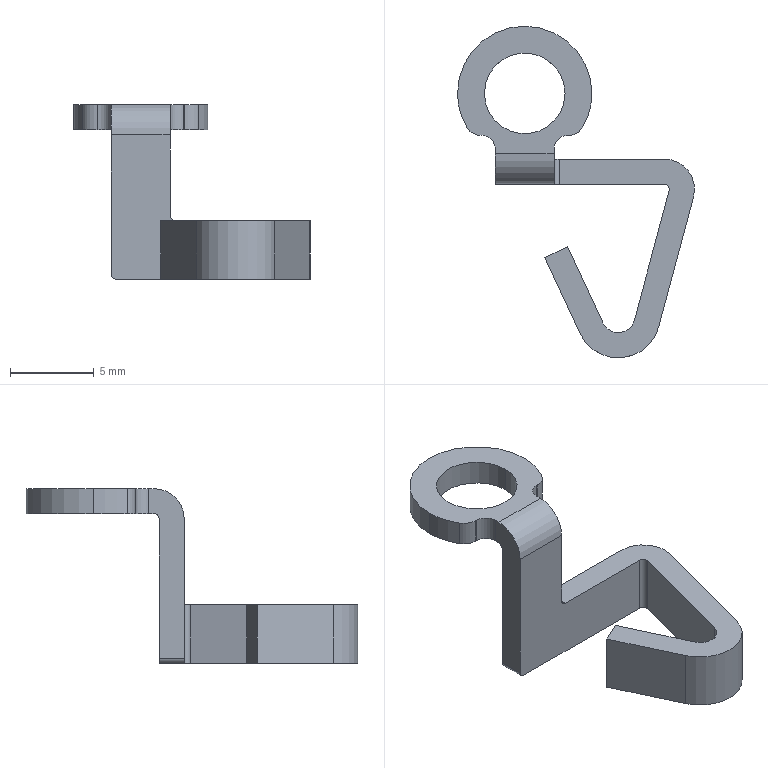Part | STEP file | TQ-DD-1105-THTerminalF1010_デフォルト | 1 solid | 32 faces | box 14.108 x 19.733 x 10.4 mm | volume 233.484 mm3 | cylinder 17 | plane 15 | commonest cylinder face diameters 0.6 x4 2 x3 8 x3 1.6 x2 3.6 x2 4.8 x2
STEP:
#1=CARTESIAN_POINT('',(2.4,0.,0.));
#2=VERTEX_POINT('',#1);
#3=CARTESIAN_POINT('',(-2.4,0.,0.));
#4=VERTEX_POINT('',#3);
#5=CARTESIAN_POINT('',(0.,0.,0.));
#6=DIRECTION('',(0.,0.,-1.));
#7=DIRECTION('',(1.,0.,0.));
#8=AXIS2_PLACEMENT_3D('',#5,#6,#7);
#9=CIRCLE('',#8,2.4);
#10=EDGE_CURVE('',#2,#4,#9,.T.);
#11=ORIENTED_EDGE('',*,*,#10,.T.);
#12=CARTESIAN_POINT('',(-2.4,0.,1.5));
#13=VERTEX_POINT('',#12);
#14=CARTESIAN_POINT('',(-2.4,0.,0.75));
#15=DIRECTION('',(0.,0.,1.));
#16=VECTOR('',#15,1000.);
#17=LINE('',#14,#16);
#18=EDGE_CURVE('',#4,#13,#17,.T.);
#19=ORIENTED_EDGE('',*,*,#18,.T.);
#20=CARTESIAN_POINT('',(2.4,0.,1.5));
#21=VERTEX_POINT('',#20);
#22=CARTESIAN_POINT('',(0.,0.,1.5));
#23=DIRECTION('',(0.,0.,-1.));
#24=DIRECTION('',(1.,0.,0.));
#25=AXIS2_PLACEMENT_3D('',#22,#23,#24);
#26=CIRCLE('',#25,2.4);
#27=EDGE_CURVE('',#21,#13,#26,.T.);
#28=ORIENTED_EDGE('',*,*,#27,.F.);
#29=CARTESIAN_POINT('',(2.4,0.,0.75));
#30=DIRECTION('',(0.,0.,1.));
#31=VECTOR('',#30,1000.);
#32=LINE('',#29,#31);
#33=EDGE_CURVE('',#2,#21,#32,.T.);
#34=ORIENTED_EDGE('',*,*,#33,.F.);
#35=EDGE_LOOP('',(#11,#19,#28,#34));
#36=FACE_OUTER_BOUND('',#35,.T.);
#37=CARTESIAN_POINT('',(0.,0.,0.75));
#38=DIRECTION('',(0.,0.,1.));
#39=DIRECTION('',(1.,0.,0.));
#40=AXIS2_PLACEMENT_3D('',#37,#38,#39);
#41=CYLINDRICAL_SURFACE('',#40,2.4);
#42=ADVANCED_FACE('',(#36),#41,.F.);
#43=CARTESIAN_POINT('',(4.,0.,0.));
#44=VERTEX_POINT('',#43);
#45=CARTESIAN_POINT('',(-4.,0.,0.));
#46=VERTEX_POINT('',#45);
#47=CARTESIAN_POINT('',(0.,0.,0.));
#48=DIRECTION('',(0.,0.,1.));
#49=DIRECTION('',(1.,0.,0.));
#50=AXIS2_PLACEMENT_3D('',#47,#48,#49);
#51=CIRCLE('',#50,4.);
#52=EDGE_CURVE('',#44,#46,#51,.T.);
#53=ORIENTED_EDGE('',*,*,#52,.T.);
#54=CARTESIAN_POINT('',(-4.,0.,1.5));
#55=VERTEX_POINT('',#54);
#56=CARTESIAN_POINT('',(-4.,0.,0.75));
#57=DIRECTION('',(0.,0.,1.));
#58=VECTOR('',#57,1000.);
#59=LINE('',#56,#58);
#60=EDGE_CURVE('',#46,#55,#59,.T.);
#61=ORIENTED_EDGE('',*,*,#60,.T.);
#62=CARTESIAN_POINT('',(4.,0.,1.5));
#63=VERTEX_POINT('',#62);
#64=CARTESIAN_POINT('',(0.,0.,1.5));
#65=DIRECTION('',(0.,0.,1.));
#66=DIRECTION('',(1.,0.,0.));
#67=AXIS2_PLACEMENT_3D('',#64,#65,#66);
#68=CIRCLE('',#67,4.);
#69=EDGE_CURVE('',#63,#55,#68,.T.);
#70=ORIENTED_EDGE('',*,*,#69,.F.);
#71=CARTESIAN_POINT('',(4.,0.,0.75));
#72=DIRECTION('',(0.,0.,1.));
#73=VECTOR('',#72,1000.);
#74=LINE('',#71,#73);
#75=EDGE_CURVE('',#44,#63,#74,.T.);
#76=ORIENTED_EDGE('',*,*,#75,.F.);
#77=EDGE_LOOP('',(#53,#61,#70,#76));
#78=FACE_OUTER_BOUND('',#77,.T.);
#79=CARTESIAN_POINT('',(0.,0.,0.75));
#80=DIRECTION('',(0.,0.,1.));
#81=DIRECTION('',(1.,0.,0.));
#82=AXIS2_PLACEMENT_3D('',#79,#80,#81);
#83=CYLINDRICAL_SURFACE('',#82,4.);
#84=ADVANCED_FACE('',(#78),#83,.T.);
#85=CARTESIAN_POINT('',(3.464,-2.,0.));
#86=VERTEX_POINT('',#85);
#87=CARTESIAN_POINT('',(0.,0.,0.));
#88=DIRECTION('',(0.,0.,1.));
#89=DIRECTION('',(1.,0.,0.));
#90=AXIS2_PLACEMENT_3D('',#87,#88,#89);
#91=CIRCLE('',#90,4.);
#92=EDGE_CURVE('',#86,#44,#91,.T.);
#93=ORIENTED_EDGE('',*,*,#92,.T.);
#94=ORIENTED_EDGE('',*,*,#75,.T.);
#95=CARTESIAN_POINT('',(3.464,-2.,1.5));
#96=VERTEX_POINT('',#95);
#97=CARTESIAN_POINT('',(0.,0.,1.5));
#98=DIRECTION('',(0.,0.,1.));
#99=DIRECTION('',(1.,0.,0.));
#100=AXIS2_PLACEMENT_3D('',#97,#98,#99);
#101=CIRCLE('',#100,4.);
#102=EDGE_CURVE('',#96,#63,#101,.T.);
#103=ORIENTED_EDGE('',*,*,#102,.F.);
#104=CARTESIAN_POINT('',(3.464,-2.,0.75));
#105=DIRECTION('',(0.,0.,1.));
#106=VECTOR('',#105,1000.);
#107=LINE('',#104,#106);
#108=EDGE_CURVE('',#86,#96,#107,.T.);
#109=ORIENTED_EDGE('',*,*,#108,.F.);
#110=EDGE_LOOP('',(#93,#94,#103,#109));
#111=FACE_OUTER_BOUND('',#110,.T.);
#112=CARTESIAN_POINT('',(0.,0.,0.75));
#113=DIRECTION('',(0.,0.,1.));
#114=DIRECTION('',(1.,0.,0.));
#115=AXIS2_PLACEMENT_3D('',#112,#113,#114);
#116=CYLINDRICAL_SURFACE('',#115,4.);
#117=ADVANCED_FACE('',(#111),#116,.T.);
#118=CARTESIAN_POINT('',(-1.75,-3.9,-0.3));
#119=VERTEX_POINT('',#118);
#120=CARTESIAN_POINT('',(-1.75,-3.9,-8.6));
#121=VERTEX_POINT('',#120);
#122=CARTESIAN_POINT('',(-1.75,-3.9,1.5));
#123=DIRECTION('',(0.,0.,-1.));
#124=VECTOR('',#123,1000.);
#125=LINE('',#122,#124);
#126=EDGE_CURVE('',#119,#121,#125,.T.);
#127=ORIENTED_EDGE('',*,*,#126,.F.);
#128=CARTESIAN_POINT('',(1.75,-3.9,-0.3));
#129=VERTEX_POINT('',#128);
#130=CARTESIAN_POINT('',(0.,-3.9,-0.3));
#131=DIRECTION('',(-1.,0.,0.));
#132=VECTOR('',#131,1000.);
#133=LINE('',#130,#132);
#134=EDGE_CURVE('',#129,#119,#133,.T.);
#135=ORIENTED_EDGE('',*,*,#134,.F.);
#136=CARTESIAN_POINT('',(1.75,-3.9,-5.1));
#137=VERTEX_POINT('',#136);
#138=CARTESIAN_POINT('',(1.75,-3.9,1.5));
#139=DIRECTION('',(0.,0.,1.));
#140=VECTOR('',#139,1000.);
#141=LINE('',#138,#140);
#142=EDGE_CURVE('',#137,#129,#141,.T.);
#143=ORIENTED_EDGE('',*,*,#142,.F.);
#144=CARTESIAN_POINT('',(2.05,-3.9,-5.4));
#145=VERTEX_POINT('',#144);
#146=CARTESIAN_POINT('',(2.05,-3.9,-5.1));
#147=DIRECTION('',(0.,-1.,0.));
#148=DIRECTION('',(0.,0.,1.));
#149=AXIS2_PLACEMENT_3D('',#146,#147,#148);
#150=CIRCLE('',#149,0.3);
#151=EDGE_CURVE('',#137,#145,#150,.T.);
#152=ORIENTED_EDGE('',*,*,#151,.T.);
#153=CARTESIAN_POINT('',(8.308,-3.9,-5.4));
#154=VERTEX_POINT('',#153);
#155=CARTESIAN_POINT('',(0.,-3.9,-5.4));
#156=DIRECTION('',(-1.,0.,0.));
#157=VECTOR('',#156,1000.);
#158=LINE('',#155,#157);
#159=EDGE_CURVE('',#154,#145,#158,.T.);
#160=ORIENTED_EDGE('',*,*,#159,.F.);
#161=CARTESIAN_POINT('',(8.308,-3.9,-8.9));
#162=VERTEX_POINT('',#161);
#163=CARTESIAN_POINT('',(8.308,-3.9,1.5));
#164=DIRECTION('',(0.,0.,1.));
#165=VECTOR('',#164,1000.);
#166=LINE('',#163,#165);
#167=EDGE_CURVE('',#162,#154,#166,.T.);
#168=ORIENTED_EDGE('',*,*,#167,.F.);
#169=CARTESIAN_POINT('',(-1.45,-3.9,-8.9));
#170=VERTEX_POINT('',#169);
#171=CARTESIAN_POINT('',(0.,-3.9,-8.9));
#172=DIRECTION('',(1.,0.,0.));
#173=VECTOR('',#172,1000.);
#174=LINE('',#171,#173);
#175=EDGE_CURVE('',#170,#162,#174,.T.);
#176=ORIENTED_EDGE('',*,*,#175,.F.);
#177=CARTESIAN_POINT('',(-1.45,-3.9,-8.6));
#178=DIRECTION('',(0.,-1.,0.));
#179=DIRECTION('',(0.,0.,1.));
#180=AXIS2_PLACEMENT_3D('',#177,#178,#179);
#181=CIRCLE('',#180,0.3);
#182=EDGE_CURVE('',#121,#170,#181,.T.);
#183=ORIENTED_EDGE('',*,*,#182,.F.);
#184=EDGE_LOOP('',(#127,#135,#143,#152,#160,#168,#176,#183));
#185=FACE_OUTER_BOUND('',#184,.T.);
#186=CARTESIAN_POINT('',(0.,-3.9,1.5));
#187=DIRECTION('',(0.,-1.,0.));
#188=DIRECTION('',(0.,0.,-1.));
#189=AXIS2_PLACEMENT_3D('',#186,#187,#188);
#190=PLANE('',#189);
#191=ADVANCED_FACE('',(#185),#190,.F.);
#192=ORIENTED_EDGE('',*,*,#126,.T.);
#193=CARTESIAN_POINT('',(-1.75,-5.4,-8.6));
#194=VERTEX_POINT('',#193);
#195=CARTESIAN_POINT('',(-1.75,-2.5,-8.6));
#196=DIRECTION('',(0.,-1.,0.));
#197=VECTOR('',#196,1000.);
#198=LINE('',#195,#197);
#199=EDGE_CURVE('',#121,#194,#198,.T.);
#200=ORIENTED_EDGE('',*,*,#199,.T.);
#201=CARTESIAN_POINT('',(-1.75,-5.4,-0.3));
#202=VERTEX_POINT('',#201);
#203=CARTESIAN_POINT('',(-1.75,-5.4,0.));
#204=DIRECTION('',(0.,0.,1.));
#205=VECTOR('',#204,1000.);
#206=LINE('',#203,#205);
#207=EDGE_CURVE('',#194,#202,#206,.T.);
#208=ORIENTED_EDGE('',*,*,#207,.T.);
#209=CARTESIAN_POINT('',(-1.75,-3.6,1.5));
#210=VERTEX_POINT('',#209);
#211=CARTESIAN_POINT('',(-1.75,-3.6,-0.3));
#212=DIRECTION('',(-1.,0.,0.));
#213=DIRECTION('',(0.,0.,-1.));
#214=AXIS2_PLACEMENT_3D('',#211,#212,#213);
#215=CIRCLE('',#214,1.8);
#216=EDGE_CURVE('',#202,#210,#215,.T.);
#217=ORIENTED_EDGE('',*,*,#216,.T.);
#218=CARTESIAN_POINT('',(-1.75,-3.3,1.5));
#219=VERTEX_POINT('',#218);
#220=CARTESIAN_POINT('',(-1.75,0.,1.5));
#221=DIRECTION('',(0.,-1.,0.));
#222=VECTOR('',#221,1000.);
#223=LINE('',#220,#222);
#224=EDGE_CURVE('',#219,#210,#223,.T.);
#225=ORIENTED_EDGE('',*,*,#224,.F.);
#226=CARTESIAN_POINT('',(-1.75,-3.3,0.));
#227=VERTEX_POINT('',#226);
#228=CARTESIAN_POINT('',(-1.75,-3.3,0.));
#229=DIRECTION('',(0.,0.,-1.));
#230=VECTOR('',#229,1000.);
#231=LINE('',#228,#230);
#232=EDGE_CURVE('',#219,#227,#231,.T.);
#233=ORIENTED_EDGE('',*,*,#232,.T.);
#234=CARTESIAN_POINT('',(-1.75,-3.6,0.));
#235=VERTEX_POINT('',#234);
#236=CARTESIAN_POINT('',(-1.75,0.,0.));
#237=DIRECTION('',(0.,-1.,0.));
#238=VECTOR('',#237,1000.);
#239=LINE('',#236,#238);
#240=EDGE_CURVE('',#227,#235,#239,.T.);
#241=ORIENTED_EDGE('',*,*,#240,.T.);
#242=CARTESIAN_POINT('',(-1.75,-3.6,-0.3));
#243=DIRECTION('',(1.,0.,0.));
#244=DIRECTION('',(0.,0.,1.));
#245=AXIS2_PLACEMENT_3D('',#242,#243,#244);
#246=CIRCLE('',#245,0.3);
#247=EDGE_CURVE('',#235,#119,#246,.T.);
#248=ORIENTED_EDGE('',*,*,#247,.T.);
#249=EDGE_LOOP('',(#192,#200,#208,#217,#225,#233,#241,#248));
#250=FACE_OUTER_BOUND('',#249,.T.);
#251=CARTESIAN_POINT('',(-1.75,-2.5,0.));
#252=DIRECTION('',(-1.,0.,0.));
#253=DIRECTION('',(0.,0.,1.));
#254=AXIS2_PLACEMENT_3D('',#251,#252,#253);
#255=PLANE('',#254);
#256=ADVANCED_FACE('',(#250),#255,.T.);
#257=ORIENTED_EDGE('',*,*,#247,.F.);
#258=CARTESIAN_POINT('',(1.75,-3.6,0.));
#259=VERTEX_POINT('',#258);
#260=CARTESIAN_POINT('',(0.,-3.6,0.));
#261=DIRECTION('',(-1.,0.,0.));
#262=VECTOR('',#261,1000.);
#263=LINE('',#260,#262);
#264=EDGE_CURVE('',#259,#235,#263,.T.);
#265=ORIENTED_EDGE('',*,*,#264,.F.);
#266=CARTESIAN_POINT('',(1.75,-3.6,-0.3));
#267=DIRECTION('',(-1.,0.,0.));
#268=DIRECTION('',(0.,0.,1.));
#269=AXIS2_PLACEMENT_3D('',#266,#267,#268);
#270=CIRCLE('',#269,0.3);
#271=EDGE_CURVE('',#129,#259,#270,.T.);
#272=ORIENTED_EDGE('',*,*,#271,.F.);
#273=ORIENTED_EDGE('',*,*,#134,.T.);
#274=EDGE_LOOP('',(#257,#265,#272,#273));
#275=FACE_OUTER_BOUND('',#274,.T.);
#276=CARTESIAN_POINT('',(0.,-3.6,-0.3));
#277=DIRECTION('',(-1.,0.,0.));
#278=DIRECTION('',(0.,0.,1.));
#279=AXIS2_PLACEMENT_3D('',#276,#277,#278);
#280=CYLINDRICAL_SURFACE('',#279,0.3);
#281=ADVANCED_FACE('',(#275),#280,.F.);
#282=CARTESIAN_POINT('',(1.75,-5.4,-0.3));
#283=VERTEX_POINT('',#282);
#284=CARTESIAN_POINT('',(1.75,-5.4,-5.1));
#285=VERTEX_POINT('',#284);
#286=CARTESIAN_POINT('',(1.75,-5.4,0.));
#287=DIRECTION('',(0.,0.,-1.));
#288=VECTOR('',#287,1000.);
#289=LINE('',#286,#288);
#290=EDGE_CURVE('',#283,#285,#289,.T.);
#291=ORIENTED_EDGE('',*,*,#290,.T.);
#292=CARTESIAN_POINT('',(1.75,-5.4,-5.1));
#293=DIRECTION('',(0.,1.,0.));
#294=VECTOR('',#293,1000.);
#295=LINE('',#292,#294);
#296=EDGE_CURVE('',#285,#137,#295,.T.);
#297=ORIENTED_EDGE('',*,*,#296,.T.);
#298=ORIENTED_EDGE('',*,*,#142,.T.);
#299=ORIENTED_EDGE('',*,*,#271,.T.);
#300=CARTESIAN_POINT('',(1.75,-3.3,0.));
#301=VERTEX_POINT('',#300);
#302=CARTESIAN_POINT('',(1.75,-5.4,0.));
#303=DIRECTION('',(0.,1.,0.));
#304=VECTOR('',#303,1000.);
#305=LINE('',#302,#304);
#306=EDGE_CURVE('',#259,#301,#305,.T.);
#307=ORIENTED_EDGE('',*,*,#306,.T.);
#308=CARTESIAN_POINT('',(1.75,-3.3,1.5));
#309=VERTEX_POINT('',#308);
#310=CARTESIAN_POINT('',(1.75,-3.3,0.));
#311=DIRECTION('',(0.,0.,1.));
#312=VECTOR('',#311,1000.);
#313=LINE('',#310,#312);
#314=EDGE_CURVE('',#301,#309,#313,.T.);
#315=ORIENTED_EDGE('',*,*,#314,.T.);
#316=CARTESIAN_POINT('',(1.75,-3.6,1.5));
#317=VERTEX_POINT('',#316);
#318=CARTESIAN_POINT('',(1.75,0.,1.5));
#319=DIRECTION('',(0.,1.,0.));
#320=VECTOR('',#319,1000.);
#321=LINE('',#318,#320);
#322=EDGE_CURVE('',#317,#309,#321,.T.);
#323=ORIENTED_EDGE('',*,*,#322,.F.);
#324=CARTESIAN_POINT('',(1.75,-3.6,-0.3));
#325=DIRECTION('',(1.,0.,0.));
#326=DIRECTION('',(0.,0.,-1.));
#327=AXIS2_PLACEMENT_3D('',#324,#325,#326);
#328=CIRCLE('',#327,1.8);
#329=EDGE_CURVE('',#317,#283,#328,.T.);
#330=ORIENTED_EDGE('',*,*,#329,.T.);
#331=EDGE_LOOP('',(#291,#297,#298,#299,#307,#315,#323,#330));
#332=FACE_OUTER_BOUND('',#331,.T.);
#333=CARTESIAN_POINT('',(1.75,-5.4,0.));
#334=DIRECTION('',(1.,0.,0.));
#335=DIRECTION('',(0.,0.,-1.));
#336=AXIS2_PLACEMENT_3D('',#333,#334,#335);
#337=PLANE('',#336);
#338=ADVANCED_FACE('',(#332),#337,.T.);
#339=CARTESIAN_POINT('',(8.308,-5.4,-5.4));
#340=VERTEX_POINT('',#339);
#341=CARTESIAN_POINT('',(2.05,-5.4,-5.4));
#342=VERTEX_POINT('',#341);
#343=CARTESIAN_POINT('',(0.,-5.4,-5.4));
#344=DIRECTION('',(-1.,0.,0.));
#345=VECTOR('',#344,1000.);
#346=LINE('',#343,#345);
#347=EDGE_CURVE('',#340,#342,#346,.T.);
#348=ORIENTED_EDGE('',*,*,#347,.F.);
#349=CARTESIAN_POINT('',(8.597,-5.778,-5.4));
#350=VERTEX_POINT('',#349);
#351=CARTESIAN_POINT('',(8.308,-5.7,-5.4));
#352=DIRECTION('',(0.,0.,-1.));
#353=DIRECTION('',(-1.,0.,0.));
#354=AXIS2_PLACEMENT_3D('',#351,#352,#353);
#355=CIRCLE('',#354,0.3);
#356=EDGE_CURVE('',#340,#350,#355,.T.);
#357=ORIENTED_EDGE('',*,*,#356,.T.);
#358=CARTESIAN_POINT('',(6.53,-13.491,-5.4));
#359=VERTEX_POINT('',#358);
#360=CARTESIAN_POINT('',(6.53,-13.491,-5.4));
#361=DIRECTION('',(0.2588,0.9659,0.));
#362=VECTOR('',#361,1000.);
#363=LINE('',#360,#362);
#364=EDGE_CURVE('',#359,#350,#363,.T.);
#365=ORIENTED_EDGE('',*,*,#364,.F.);
#366=CARTESIAN_POINT('',(4.658,-13.655,-5.4));
#367=VERTEX_POINT('',#366);
#368=CARTESIAN_POINT('',(5.565,-13.233,-5.4));
#369=DIRECTION('',(0.,0.,1.));
#370=DIRECTION('',(-1.,0.,0.));
#371=AXIS2_PLACEMENT_3D('',#368,#369,#370);
#372=CIRCLE('',#371,1.);
#373=EDGE_CURVE('',#367,#359,#372,.T.);
#374=ORIENTED_EDGE('',*,*,#373,.F.);
#375=CARTESIAN_POINT('',(2.545,-9.124,-5.4));
#376=VERTEX_POINT('',#375);
#377=CARTESIAN_POINT('',(2.545,-9.124,-5.4));
#378=DIRECTION('',(0.4226,-0.9063,0.));
#379=VECTOR('',#378,1000.);
#380=LINE('',#377,#379);
#381=EDGE_CURVE('',#376,#367,#380,.T.);
#382=ORIENTED_EDGE('',*,*,#381,.F.);
#383=CARTESIAN_POINT('',(1.186,-9.758,-5.4));
#384=VERTEX_POINT('',#383);
#385=CARTESIAN_POINT('',(2.545,-9.124,-5.4));
#386=DIRECTION('',(0.9063,0.4226,0.));
#387=VECTOR('',#386,1000.);
#388=LINE('',#385,#387);
#389=EDGE_CURVE('',#384,#376,#388,.T.);
#390=ORIENTED_EDGE('',*,*,#389,.F.);
#391=CARTESIAN_POINT('',(3.299,-14.289,-5.4));
#392=VERTEX_POINT('',#391);
#393=CARTESIAN_POINT('',(3.299,-14.289,-5.4));
#394=DIRECTION('',(-0.4226,0.9063,0.));
#395=VECTOR('',#394,1000.);
#396=LINE('',#393,#395);
#397=EDGE_CURVE('',#392,#384,#396,.T.);
#398=ORIENTED_EDGE('',*,*,#397,.F.);
#399=CARTESIAN_POINT('',(7.979,-13.88,-5.4));
#400=VERTEX_POINT('',#399);
#401=CARTESIAN_POINT('',(5.565,-13.233,-5.4));
#402=DIRECTION('',(0.,0.,-1.));
#403=DIRECTION('',(-1.,0.,0.));
#404=AXIS2_PLACEMENT_3D('',#401,#402,#403);
#405=CIRCLE('',#404,2.5);
#406=EDGE_CURVE('',#400,#392,#405,.T.);
#407=ORIENTED_EDGE('',*,*,#406,.F.);
#408=CARTESIAN_POINT('',(10.046,-6.166,-5.4));
#409=VERTEX_POINT('',#408);
#410=CARTESIAN_POINT('',(10.046,-6.166,-5.4));
#411=DIRECTION('',(-0.2588,-0.9659,0.));
#412=VECTOR('',#411,1000.);
#413=LINE('',#410,#412);
#414=EDGE_CURVE('',#409,#400,#413,.T.);
#415=ORIENTED_EDGE('',*,*,#414,.F.);
#416=CARTESIAN_POINT('',(8.308,-5.7,-5.4));
#417=DIRECTION('',(0.,0.,-1.));
#418=DIRECTION('',(-1.,0.,0.));
#419=AXIS2_PLACEMENT_3D('',#416,#417,#418);
#420=CIRCLE('',#419,1.8);
#421=EDGE_CURVE('',#154,#409,#420,.T.);
#422=ORIENTED_EDGE('',*,*,#421,.F.);
#423=ORIENTED_EDGE('',*,*,#159,.T.);
#424=CARTESIAN_POINT('',(2.05,0.,-5.4));
#425=DIRECTION('',(0.,1.,0.));
#426=VECTOR('',#425,1000.);
#427=LINE('',#424,#426);
#428=EDGE_CURVE('',#342,#145,#427,.T.);
#429=ORIENTED_EDGE('',*,*,#428,.F.);
#430=EDGE_LOOP('',(#348,#357,#365,#374,#382,#390,#398,#407,#415,#422,#423,#429));
#431=FACE_OUTER_BOUND('',#430,.T.);
#432=CARTESIAN_POINT('',(0.,0.,-5.4));
#433=DIRECTION('',(0.,0.,-1.));
#434=DIRECTION('',(-1.,0.,0.));
#435=AXIS2_PLACEMENT_3D('',#432,#433,#434);
#436=PLANE('',#435);
#437=ADVANCED_FACE('',(#431),#436,.F.);
#438=CARTESIAN_POINT('',(10.046,-6.166,-8.9));
#439=VERTEX_POINT('',#438);
#440=CARTESIAN_POINT('',(8.308,-5.7,-8.9));
#441=DIRECTION('',(0.,0.,1.));
#442=DIRECTION('',(-1.,0.,0.));
#443=AXIS2_PLACEMENT_3D('',#440,#441,#442);
#444=CIRCLE('',#443,1.8);
#445=EDGE_CURVE('',#439,#162,#444,.T.);
#446=ORIENTED_EDGE('',*,*,#445,.T.);
#447=ORIENTED_EDGE('',*,*,#167,.T.);
#448=ORIENTED_EDGE('',*,*,#421,.T.);
#449=CARTESIAN_POINT('',(10.046,-6.166,-7.15));
#450=DIRECTION('',(0.,0.,-1.));
#451=VECTOR('',#450,1000.);
#452=LINE('',#449,#451);
#453=EDGE_CURVE('',#409,#439,#452,.T.);
#454=ORIENTED_EDGE('',*,*,#453,.T.);
#455=EDGE_LOOP('',(#446,#447,#448,#454));
#456=FACE_OUTER_BOUND('',#455,.T.);
#457=CARTESIAN_POINT('',(8.308,-5.7,-7.15));
#458=DIRECTION('',(0.,0.,-1.));
#459=DIRECTION('',(-1.,0.,0.));
#460=AXIS2_PLACEMENT_3D('',#457,#458,#459);
#461=CYLINDRICAL_SURFACE('',#460,1.8);
#462=ADVANCED_FACE('',(#456),#461,.T.);
#463=CARTESIAN_POINT('',(8.308,-5.4,-8.9));
#464=VERTEX_POINT('',#463);
#465=CARTESIAN_POINT('',(-1.45,-5.4,-8.9));
#466=VERTEX_POINT('',#465);
#467=CARTESIAN_POINT('',(0.,-5.4,-8.9));
#468=DIRECTION('',(-1.,0.,0.));
#469=VECTOR('',#468,1000.);
#470=LINE('',#467,#469);
#471=EDGE_CURVE('',#464,#466,#470,.T.);
#472=ORIENTED_EDGE('',*,*,#471,.T.);
#473=CARTESIAN_POINT('',(-1.45,-5.4,-8.9));
#474=DIRECTION('',(0.,1.,0.));
#475=VECTOR('',#474,1000.);
#476=LINE('',#473,#475);
#477=EDGE_CURVE('',#466,#170,#476,.T.);
#478=ORIENTED_EDGE('',*,*,#477,.T.);
#479=ORIENTED_EDGE('',*,*,#175,.T.);
#480=ORIENTED_EDGE('',*,*,#445,.F.);
#481=CARTESIAN_POINT('',(7.979,-13.88,-8.9));
#482=VERTEX_POINT('',#481);
#483=CARTESIAN_POINT('',(10.046,-6.166,-8.9));
#484=DIRECTION('',(-0.2588,-0.9659,0.));
#485=VECTOR('',#484,1000.);
#486=LINE('',#483,#485);
#487=EDGE_CURVE('',#439,#482,#486,.T.);
#488=ORIENTED_EDGE('',*,*,#487,.T.);
#489=CARTESIAN_POINT('',(3.299,-14.289,-8.9));
#490=VERTEX_POINT('',#489);
#491=CARTESIAN_POINT('',(5.565,-13.233,-8.9));
#492=DIRECTION('',(0.,0.,-1.));
#493=DIRECTION('',(-1.,0.,0.));
#494=AXIS2_PLACEMENT_3D('',#491,#492,#493);
#495=CIRCLE('',#494,2.5);
#496=EDGE_CURVE('',#482,#490,#495,.T.);
#497=ORIENTED_EDGE('',*,*,#496,.T.);
#498=CARTESIAN_POINT('',(1.186,-9.758,-8.9));
#499=VERTEX_POINT('',#498);
#500=CARTESIAN_POINT('',(3.299,-14.289,-8.9));
#501=DIRECTION('',(-0.4226,0.9063,0.));
#502=VECTOR('',#501,1000.);
#503=LINE('',#500,#502);
#504=EDGE_CURVE('',#490,#499,#503,.T.);
#505=ORIENTED_EDGE('',*,*,#504,.T.);
#506=CARTESIAN_POINT('',(2.545,-9.124,-8.9));
#507=VERTEX_POINT('',#506);
#508=CARTESIAN_POINT('',(2.545,-9.124,-8.9));
#509=DIRECTION('',(-0.9063,-0.4226,0.));
#510=VECTOR('',#509,1000.);
#511=LINE('',#508,#510);
#512=EDGE_CURVE('',#507,#499,#511,.T.);
#513=ORIENTED_EDGE('',*,*,#512,.F.);
#514=CARTESIAN_POINT('',(4.658,-13.655,-8.9));
#515=VERTEX_POINT('',#514);
#516=CARTESIAN_POINT('',(2.545,-9.124,-8.9));
#517=DIRECTION('',(0.4226,-0.9063,0.));
#518=VECTOR('',#517,1000.);
#519=LINE('',#516,#518);
#520=EDGE_CURVE('',#507,#515,#519,.T.);
#521=ORIENTED_EDGE('',*,*,#520,.T.);
#522=CARTESIAN_POINT('',(6.53,-13.491,-8.9));
#523=VERTEX_POINT('',#522);
#524=CARTESIAN_POINT('',(5.565,-13.233,-8.9));
#525=DIRECTION('',(0.,0.,1.));
#526=DIRECTION('',(-1.,0.,0.));
#527=AXIS2_PLACEMENT_3D('',#524,#525,#526);
#528=CIRCLE('',#527,1.);
#529=EDGE_CURVE('',#515,#523,#528,.T.);
#530=ORIENTED_EDGE('',*,*,#529,.T.);
#531=CARTESIAN_POINT('',(8.597,-5.778,-8.9));
#532=VERTEX_POINT('',#531);
#533=CARTESIAN_POINT('',(6.53,-13.491,-8.9));
#534=DIRECTION('',(0.2588,0.9659,0.));
#535=VECTOR('',#534,1000.);
#536=LINE('',#533,#535);
#537=EDGE_CURVE('',#523,#532,#536,.T.);
#538=ORIENTED_EDGE('',*,*,#537,.T.);
#539=CARTESIAN_POINT('',(8.308,-5.7,-8.9));
#540=DIRECTION('',(0.,0.,1.));
#541=DIRECTION('',(-1.,0.,0.));
#542=AXIS2_PLACEMENT_3D('',#539,#540,#541);
#543=CIRCLE('',#542,0.3);
#544=EDGE_CURVE('',#532,#464,#543,.T.);
#545=ORIENTED_EDGE('',*,*,#544,.T.);
#546=EDGE_LOOP('',(#472,#478,#479,#480,#488,#497,#505,#513,#521,#530,#538,#545));
#547=FACE_OUTER_BOUND('',#546,.T.);
#548=CARTESIAN_POINT('',(0.,-5.4,-8.9));
#549=DIRECTION('',(0.,0.,-1.));
#550=DIRECTION('',(-1.,0.,0.));
#551=AXIS2_PLACEMENT_3D('',#548,#549,#550);
#552=PLANE('',#551);
#553=ADVANCED_FACE('',(#547),#552,.T.);
#554=CARTESIAN_POINT('',(-1.45,-5.4,-8.6));
#555=DIRECTION('',(0.,1.,0.));
#556=DIRECTION('',(0.,0.,1.));
#557=AXIS2_PLACEMENT_3D('',#554,#555,#556);
#558=CIRCLE('',#557,0.3);
#559=EDGE_CURVE('',#466,#194,#558,.T.);
#560=ORIENTED_EDGE('',*,*,#559,.T.);
#561=ORIENTED_EDGE('',*,*,#199,.F.);
#562=ORIENTED_EDGE('',*,*,#182,.T.);
#563=ORIENTED_EDGE('',*,*,#477,.F.);
#564=EDGE_LOOP('',(#560,#561,#562,#563));
#565=FACE_OUTER_BOUND('',#564,.T.);
#566=CARTESIAN_POINT('',(-1.45,-9.816,-8.6));
#567=DIRECTION('',(0.,1.,0.));
#568=DIRECTION('',(0.,0.,1.));
#569=AXIS2_PLACEMENT_3D('',#566,#567,#568);
#570=CYLINDRICAL_SURFACE('',#569,0.3);
#571=ADVANCED_FACE('',(#565),#570,.T.);
#572=CARTESIAN_POINT('',(-2.55,-2.5,1.5));
#573=VERTEX_POINT('',#572);
#574=CARTESIAN_POINT('',(-2.55,-3.3,1.5));
#575=DIRECTION('',(0.,0.,-1.));
#576=DIRECTION('',(1.,0.,0.));
#577=AXIS2_PLACEMENT_3D('',#574,#575,#576);
#578=CIRCLE('',#577,0.8);
#579=EDGE_CURVE('',#573,#219,#578,.T.);
#580=ORIENTED_EDGE('',*,*,#579,.F.);
#581=CARTESIAN_POINT('',(-2.55,-2.5,0.));
#582=VERTEX_POINT('',#581);
#583=CARTESIAN_POINT('',(-2.55,-2.5,-3.7));
#584=DIRECTION('',(0.,0.,1.));
#585=VECTOR('',#584,1000.);
#586=LINE('',#583,#585);
#587=EDGE_CURVE('',#582,#573,#586,.T.);
#588=ORIENTED_EDGE('',*,*,#587,.F.);
#589=CARTESIAN_POINT('',(-2.55,-3.3,0.));
#590=DIRECTION('',(0.,0.,1.));
#591=DIRECTION('',(1.,0.,0.));
#592=AXIS2_PLACEMENT_3D('',#589,#590,#591);
#593=CIRCLE('',#592,0.8);
#594=EDGE_CURVE('',#227,#582,#593,.T.);
#595=ORIENTED_EDGE('',*,*,#594,.F.);
#596=ORIENTED_EDGE('',*,*,#232,.F.);
#597=EDGE_LOOP('',(#580,#588,#595,#596));
#598=FACE_OUTER_BOUND('',#597,.T.);
#599=CARTESIAN_POINT('',(-2.55,-3.3,-3.7));
#600=DIRECTION('',(0.,0.,1.));
#601=DIRECTION('',(1.,0.,0.));
#602=AXIS2_PLACEMENT_3D('',#599,#600,#601);
#603=CYLINDRICAL_SURFACE('',#602,0.8);
#604=ADVANCED_FACE('',(#598),#603,.F.);
#605=ORIENTED_EDGE('',*,*,#216,.F.);
#606=CARTESIAN_POINT('',(0.,-5.4,-0.3));
#607=DIRECTION('',(1.,0.,0.));
#608=VECTOR('',#607,1000.);
#609=LINE('',#606,#608);
#610=EDGE_CURVE('',#202,#283,#609,.T.);
#611=ORIENTED_EDGE('',*,*,#610,.T.);
#612=ORIENTED_EDGE('',*,*,#329,.F.);
#613=CARTESIAN_POINT('',(0.,-3.6,1.5));
#614=DIRECTION('',(-1.,0.,0.));
#615=VECTOR('',#614,1000.);
#616=LINE('',#613,#615);
#617=EDGE_CURVE('',#317,#210,#616,.T.);
#618=ORIENTED_EDGE('',*,*,#617,.T.);
#619=EDGE_LOOP('',(#605,#611,#612,#618));
#620=FACE_OUTER_BOUND('',#619,.T.);
#621=CARTESIAN_POINT('',(0.,-3.6,-0.3));
#622=DIRECTION('',(1.,0.,0.));
#623=DIRECTION('',(0.,0.,-1.));
#624=AXIS2_PLACEMENT_3D('',#621,#622,#623);
#625=CYLINDRICAL_SURFACE('',#624,1.8);
#626=ADVANCED_FACE('',(#620),#625,.T.);
#627=ORIENTED_EDGE('',*,*,#207,.F.);
#628=ORIENTED_EDGE('',*,*,#559,.F.);
#629=ORIENTED_EDGE('',*,*,#471,.F.);
#630=CARTESIAN_POINT('',(8.308,-5.4,0.));
#631=DIRECTION('',(0.,0.,1.));
#632=VECTOR('',#631,1000.);
#633=LINE('',#630,#632);
#634=EDGE_CURVE('',#464,#340,#633,.T.);
#635=ORIENTED_EDGE('',*,*,#634,.T.);
#636=ORIENTED_EDGE('',*,*,#347,.T.);
#637=CARTESIAN_POINT('',(2.05,-5.4,-5.1));
#638=DIRECTION('',(0.,1.,0.));
#639=DIRECTION('',(0.,0.,1.));
#640=AXIS2_PLACEMENT_3D('',#637,#638,#639);
#641=CIRCLE('',#640,0.3);
#642=EDGE_CURVE('',#342,#285,#641,.T.);
#643=ORIENTED_EDGE('',*,*,#642,.T.);
#644=ORIENTED_EDGE('',*,*,#290,.F.);
#645=ORIENTED_EDGE('',*,*,#610,.F.);
#646=EDGE_LOOP('',(#627,#628,#629,#635,#636,#643,#644,#645));
#647=FACE_OUTER_BOUND('',#646,.T.);
#648=CARTESIAN_POINT('',(-1.75,-5.4,0.));
#649=DIRECTION('',(0.,-1.,0.));
#650=DIRECTION('',(0.,0.,-1.));
#651=AXIS2_PLACEMENT_3D('',#648,#649,#650);
#652=PLANE('',#651);
#653=ADVANCED_FACE('',(#647),#652,.T.);
#654=ORIENTED_EDGE('',*,*,#10,.F.);
#655=CARTESIAN_POINT('',(0.,0.,0.));
#656=DIRECTION('',(0.,0.,-1.));
#657=DIRECTION('',(1.,0.,0.));
#658=AXIS2_PLACEMENT_3D('',#655,#656,#657);
#659=CIRCLE('',#658,2.4);
#660=EDGE_CURVE('',#4,#2,#659,.T.);
#661=ORIENTED_EDGE('',*,*,#660,.F.);
#662=EDGE_LOOP('',(#654,#661));
#663=FACE_BOUND('',#662,.T.);
#664=CARTESIAN_POINT('',(2.55,-2.5,0.));
#665=VERTEX_POINT('',#664);
#666=CARTESIAN_POINT('',(2.598,-2.5,0.));
#667=VERTEX_POINT('',#666);
#668=CARTESIAN_POINT('',(-3.122,-2.5,0.));
#669=DIRECTION('',(1.,0.,0.));
#670=VECTOR('',#669,1000.);
#671=LINE('',#668,#670);
#672=EDGE_CURVE('',#665,#667,#671,.T.);
#673=ORIENTED_EDGE('',*,*,#672,.F.);
#674=CARTESIAN_POINT('',(2.55,-3.3,0.));
#675=DIRECTION('',(0.,0.,-1.));
#676=DIRECTION('',(1.,0.,0.));
#677=AXIS2_PLACEMENT_3D('',#674,#675,#676);
#678=CIRCLE('',#677,0.8);
#679=EDGE_CURVE('',#301,#665,#678,.T.);
#680=ORIENTED_EDGE('',*,*,#679,.F.);
#681=ORIENTED_EDGE('',*,*,#306,.F.);
#682=ORIENTED_EDGE('',*,*,#264,.T.);
#683=ORIENTED_EDGE('',*,*,#240,.F.);
#684=ORIENTED_EDGE('',*,*,#594,.T.);
#685=CARTESIAN_POINT('',(-2.598,-2.5,0.));
#686=VERTEX_POINT('',#685);
#687=CARTESIAN_POINT('',(0.,-2.5,0.));
#688=DIRECTION('',(1.,0.,0.));
#689=VECTOR('',#688,1000.);
#690=LINE('',#687,#689);
#691=EDGE_CURVE('',#686,#582,#690,.T.);
#692=ORIENTED_EDGE('',*,*,#691,.F.);
#693=CARTESIAN_POINT('',(-3.464,-2.,0.));
#694=VERTEX_POINT('',#693);
#695=CARTESIAN_POINT('',(-2.598,-1.5,0.));
#696=DIRECTION('',(0.,0.,1.));
#697=DIRECTION('',(-1.,0.,0.));
#698=AXIS2_PLACEMENT_3D('',#695,#696,#697);
#699=CIRCLE('',#698,1.);
#700=EDGE_CURVE('',#694,#686,#699,.T.);
#701=ORIENTED_EDGE('',*,*,#700,.F.);
#702=CARTESIAN_POINT('',(0.,0.,0.));
#703=DIRECTION('',(0.,0.,1.));
#704=DIRECTION('',(1.,0.,0.));
#705=AXIS2_PLACEMENT_3D('',#702,#703,#704);
#706=CIRCLE('',#705,4.);
#707=EDGE_CURVE('',#46,#694,#706,.T.);
#708=ORIENTED_EDGE('',*,*,#707,.F.);
#709=ORIENTED_EDGE('',*,*,#52,.F.);
#710=ORIENTED_EDGE('',*,*,#92,.F.);
#711=CARTESIAN_POINT('',(2.598,-1.5,0.));
#712=DIRECTION('',(0.,0.,1.));
#713=DIRECTION('',(-1.,0.,0.));
#714=AXIS2_PLACEMENT_3D('',#711,#712,#713);
#715=CIRCLE('',#714,1.);
#716=EDGE_CURVE('',#667,#86,#715,.T.);
#717=ORIENTED_EDGE('',*,*,#716,.F.);
#718=EDGE_LOOP('',(#673,#680,#681,#682,#683,#684,#692,#701,#708,#709,#710,#717));
#719=FACE_OUTER_BOUND('',#718,.T.);
#720=CARTESIAN_POINT('',(0.,0.,0.));
#721=DIRECTION('',(0.,0.,1.));
#722=DIRECTION('',(1.,0.,0.));
#723=AXIS2_PLACEMENT_3D('',#720,#721,#722);
#724=PLANE('',#723);
#725=ADVANCED_FACE('',(#663,#719),#724,.F.);
#726=ORIENTED_EDGE('',*,*,#151,.F.);
#727=ORIENTED_EDGE('',*,*,#296,.F.);
#728=ORIENTED_EDGE('',*,*,#642,.F.);
#729=ORIENTED_EDGE('',*,*,#428,.T.);
#730=EDGE_LOOP('',(#726,#727,#728,#729));
#731=FACE_OUTER_BOUND('',#730,.T.);
#732=CARTESIAN_POINT('',(2.05,-9.816,-5.1));
#733=DIRECTION('',(0.,1.,0.));
#734=DIRECTION('',(0.,0.,1.));
#735=AXIS2_PLACEMENT_3D('',#732,#733,#734);
#736=CYLINDRICAL_SURFACE('',#735,0.3);
#737=ADVANCED_FACE('',(#731),#736,.F.);
#738=CARTESIAN_POINT('',(2.55,-2.5,1.5));
#739=VERTEX_POINT('',#738);
#740=CARTESIAN_POINT('',(2.55,-3.3,1.5));
#741=DIRECTION('',(0.,0.,-1.));
#742=DIRECTION('',(1.,0.,0.));
#743=AXIS2_PLACEMENT_3D('',#740,#741,#742);
#744=CIRCLE('',#743,0.8);
#745=EDGE_CURVE('',#309,#739,#744,.T.);
#746=ORIENTED_EDGE('',*,*,#745,.F.);
#747=ORIENTED_EDGE('',*,*,#314,.F.);
#748=ORIENTED_EDGE('',*,*,#679,.T.);
#749=CARTESIAN_POINT('',(2.55,-2.5,-3.7));
#750=DIRECTION('',(0.,0.,-1.));
#751=VECTOR('',#750,1000.);
#752=LINE('',#749,#751);
#753=EDGE_CURVE('',#739,#665,#752,.T.);
#754=ORIENTED_EDGE('',*,*,#753,.F.);
#755=EDGE_LOOP('',(#746,#747,#748,#754));
#756=FACE_OUTER_BOUND('',#755,.T.);
#757=CARTESIAN_POINT('',(2.55,-3.3,-3.7));
#758=DIRECTION('',(0.,0.,1.));
#759=DIRECTION('',(1.,0.,0.));
#760=AXIS2_PLACEMENT_3D('',#757,#758,#759);
#761=CYLINDRICAL_SURFACE('',#760,0.8);
#762=ADVANCED_FACE('',(#756),#761,.F.);
#763=CARTESIAN_POINT('',(8.597,-5.778,-8.9));
#764=DIRECTION('',(0.,0.,1.));
#765=VECTOR('',#764,1000.);
#766=LINE('',#763,#765);
#767=EDGE_CURVE('',#532,#350,#766,.T.);
#768=ORIENTED_EDGE('',*,*,#767,.F.);
#769=ORIENTED_EDGE('',*,*,#537,.F.);
#770=CARTESIAN_POINT('',(6.53,-13.491,-8.9));
#771=DIRECTION('',(0.,0.,-1.));
#772=VECTOR('',#771,1000.);
#773=LINE('',#770,#772);
#774=EDGE_CURVE('',#359,#523,#773,.T.);
#775=ORIENTED_EDGE('',*,*,#774,.F.);
#776=ORIENTED_EDGE('',*,*,#364,.T.);
#777=EDGE_LOOP('',(#768,#769,#775,#776));
#778=FACE_OUTER_BOUND('',#777,.T.);
#779=CARTESIAN_POINT('',(6.53,-13.491,-8.9));
#780=DIRECTION('',(0.9659,-0.2588,0.));
#781=DIRECTION('',(0.2588,0.9659,0.));
#782=AXIS2_PLACEMENT_3D('',#779,#780,#781);
#783=PLANE('',#782);
#784=ADVANCED_FACE('',(#778),#783,.F.);
#785=ORIENTED_EDGE('',*,*,#774,.T.);
#786=ORIENTED_EDGE('',*,*,#529,.F.);
#787=CARTESIAN_POINT('',(4.658,-13.655,-7.15));
#788=DIRECTION('',(0.,0.,-1.));
#789=VECTOR('',#788,1000.);
#790=LINE('',#787,#789);
#791=EDGE_CURVE('',#367,#515,#790,.T.);
#792=ORIENTED_EDGE('',*,*,#791,.F.);
#793=ORIENTED_EDGE('',*,*,#373,.T.);
#794=EDGE_LOOP('',(#785,#786,#792,#793));
#795=FACE_OUTER_BOUND('',#794,.T.);
#796=CARTESIAN_POINT('',(5.565,-13.233,-7.15));
#797=DIRECTION('',(0.,0.,-1.));
#798=DIRECTION('',(-1.,0.,0.));
#799=AXIS2_PLACEMENT_3D('',#796,#797,#798);
#800=CYLINDRICAL_SURFACE('',#799,1.);
#801=ADVANCED_FACE('',(#795),#800,.F.);
#802=ORIENTED_EDGE('',*,*,#791,.T.);
#803=ORIENTED_EDGE('',*,*,#520,.F.);
#804=CARTESIAN_POINT('',(2.545,-9.124,-8.9));
#805=DIRECTION('',(0.,0.,-1.));
#806=VECTOR('',#805,1000.);
#807=LINE('',#804,#806);
#808=EDGE_CURVE('',#376,#507,#807,.T.);
#809=ORIENTED_EDGE('',*,*,#808,.F.);
#810=ORIENTED_EDGE('',*,*,#381,.T.);
#811=EDGE_LOOP('',(#802,#803,#809,#810));
#812=FACE_OUTER_BOUND('',#811,.T.);
#813=CARTESIAN_POINT('',(2.545,-9.124,-8.9));
#814=DIRECTION('',(-0.9063,-0.4226,0.));
#815=DIRECTION('',(0.4226,-0.9063,0.));
#816=AXIS2_PLACEMENT_3D('',#813,#814,#815);
#817=PLANE('',#816);
#818=ADVANCED_FACE('',(#812),#817,.F.);
#819=ORIENTED_EDGE('',*,*,#504,.F.);
#820=CARTESIAN_POINT('',(3.299,-14.289,-8.9));
#821=DIRECTION('',(0.,0.,1.));
#822=VECTOR('',#821,1000.);
#823=LINE('',#820,#822);
#824=EDGE_CURVE('',#490,#392,#823,.T.);
#825=ORIENTED_EDGE('',*,*,#824,.T.);
#826=ORIENTED_EDGE('',*,*,#397,.T.);
#827=CARTESIAN_POINT('',(1.186,-9.758,-8.9));
#828=DIRECTION('',(0.,0.,-1.));
#829=VECTOR('',#828,1000.);
#830=LINE('',#827,#829);
#831=EDGE_CURVE('',#384,#499,#830,.T.);
#832=ORIENTED_EDGE('',*,*,#831,.T.);
#833=EDGE_LOOP('',(#819,#825,#826,#832));
#834=FACE_OUTER_BOUND('',#833,.T.);
#835=CARTESIAN_POINT('',(1.186,-9.758,-8.9));
#836=DIRECTION('',(-0.9063,-0.4226,0.));
#837=DIRECTION('',(0.4226,-0.9063,0.));
#838=AXIS2_PLACEMENT_3D('',#835,#836,#837);
#839=PLANE('',#838);
#840=ADVANCED_FACE('',(#834),#839,.T.);
#841=ORIENTED_EDGE('',*,*,#496,.F.);
#842=CARTESIAN_POINT('',(7.979,-13.88,-7.15));
#843=DIRECTION('',(0.,0.,1.));
#844=VECTOR('',#843,1000.);
#845=LINE('',#842,#844);
#846=EDGE_CURVE('',#482,#400,#845,.T.);
#847=ORIENTED_EDGE('',*,*,#846,.T.);
#848=ORIENTED_EDGE('',*,*,#406,.T.);
#849=ORIENTED_EDGE('',*,*,#824,.F.);
#850=EDGE_LOOP('',(#841,#847,#848,#849));
#851=FACE_OUTER_BOUND('',#850,.T.);
#852=CARTESIAN_POINT('',(5.565,-13.233,-7.15));
#853=DIRECTION('',(0.,0.,-1.));
#854=DIRECTION('',(-1.,0.,0.));
#855=AXIS2_PLACEMENT_3D('',#852,#853,#854);
#856=CYLINDRICAL_SURFACE('',#855,2.5);
#857=ADVANCED_FACE('',(#851),#856,.T.);
#858=ORIENTED_EDGE('',*,*,#846,.F.);
#859=ORIENTED_EDGE('',*,*,#487,.F.);
#860=ORIENTED_EDGE('',*,*,#453,.F.);
#861=ORIENTED_EDGE('',*,*,#414,.T.);
#862=EDGE_LOOP('',(#858,#859,#860,#861));
#863=FACE_OUTER_BOUND('',#862,.T.);
#864=CARTESIAN_POINT('',(10.046,-6.166,-8.9));
#865=DIRECTION('',(-0.9659,0.2588,0.));
#866=DIRECTION('',(-0.2588,-0.9659,0.));
#867=AXIS2_PLACEMENT_3D('',#864,#865,#866);
#868=PLANE('',#867);
#869=ADVANCED_FACE('',(#863),#868,.F.);
#870=CARTESIAN_POINT('',(-2.598,-2.5,1.5));
#871=VERTEX_POINT('',#870);
#872=CARTESIAN_POINT('',(-3.122,-2.5,1.5));
#873=DIRECTION('',(-1.,0.,0.));
#874=VECTOR('',#873,1000.);
#875=LINE('',#872,#874);
#876=EDGE_CURVE('',#573,#871,#875,.T.);
#877=ORIENTED_EDGE('',*,*,#876,.T.);
#878=CARTESIAN_POINT('',(-2.598,-2.5,0.));
#879=DIRECTION('',(0.,0.,-1.));
#880=VECTOR('',#879,1000.);
#881=LINE('',#878,#880);
#882=EDGE_CURVE('',#871,#686,#881,.T.);
#883=ORIENTED_EDGE('',*,*,#882,.T.);
#884=ORIENTED_EDGE('',*,*,#691,.T.);
#885=ORIENTED_EDGE('',*,*,#587,.T.);
#886=EDGE_LOOP('',(#877,#883,#884,#885));
#887=FACE_OUTER_BOUND('',#886,.T.);
#888=CARTESIAN_POINT('',(-3.122,-2.5,0.));
#889=DIRECTION('',(0.,-1.,0.));
#890=DIRECTION('',(0.,0.,-1.));
#891=AXIS2_PLACEMENT_3D('',#888,#889,#890);
#892=PLANE('',#891);
#893=ADVANCED_FACE('',(#887),#892,.T.);
#894=ORIENTED_EDGE('',*,*,#27,.T.);
#895=CARTESIAN_POINT('',(0.,0.,1.5));
#896=DIRECTION('',(0.,0.,-1.));
#897=DIRECTION('',(1.,0.,0.));
#898=AXIS2_PLACEMENT_3D('',#895,#896,#897);
#899=CIRCLE('',#898,2.4);
#900=EDGE_CURVE('',#13,#21,#899,.T.);
#901=ORIENTED_EDGE('',*,*,#900,.T.);
#902=EDGE_LOOP('',(#894,#901));
#903=FACE_BOUND('',#902,.T.);
#904=CARTESIAN_POINT('',(2.598,-2.5,1.5));
#905=VERTEX_POINT('',#904);
#906=CARTESIAN_POINT('',(0.,-2.5,1.5));
#907=DIRECTION('',(1.,0.,0.));
#908=VECTOR('',#907,1000.);
#909=LINE('',#906,#908);
#910=EDGE_CURVE('',#739,#905,#909,.T.);
#911=ORIENTED_EDGE('',*,*,#910,.T.);
#912=CARTESIAN_POINT('',(2.598,-1.5,1.5));
#913=DIRECTION('',(0.,0.,1.));
#914=DIRECTION('',(-1.,0.,0.));
#915=AXIS2_PLACEMENT_3D('',#912,#913,#914);
#916=CIRCLE('',#915,1.);
#917=EDGE_CURVE('',#905,#96,#916,.T.);
#918=ORIENTED_EDGE('',*,*,#917,.T.);
#919=ORIENTED_EDGE('',*,*,#102,.T.);
#920=ORIENTED_EDGE('',*,*,#69,.T.);
#921=CARTESIAN_POINT('',(-3.464,-2.,1.5));
#922=VERTEX_POINT('',#921);
#923=CARTESIAN_POINT('',(0.,0.,1.5));
#924=DIRECTION('',(0.,0.,1.));
#925=DIRECTION('',(1.,0.,0.));
#926=AXIS2_PLACEMENT_3D('',#923,#924,#925);
#927=CIRCLE('',#926,4.);
#928=EDGE_CURVE('',#55,#922,#927,.T.);
#929=ORIENTED_EDGE('',*,*,#928,.T.);
#930=CARTESIAN_POINT('',(-2.598,-1.5,1.5));
#931=DIRECTION('',(0.,0.,1.));
#932=DIRECTION('',(-1.,0.,0.));
#933=AXIS2_PLACEMENT_3D('',#930,#931,#932);
#934=CIRCLE('',#933,1.);
#935=EDGE_CURVE('',#922,#871,#934,.T.);
#936=ORIENTED_EDGE('',*,*,#935,.T.);
#937=ORIENTED_EDGE('',*,*,#876,.F.);
#938=ORIENTED_EDGE('',*,*,#579,.T.);
#939=ORIENTED_EDGE('',*,*,#224,.T.);
#940=ORIENTED_EDGE('',*,*,#617,.F.);
#941=ORIENTED_EDGE('',*,*,#322,.T.);
#942=ORIENTED_EDGE('',*,*,#745,.T.);
#943=EDGE_LOOP('',(#911,#918,#919,#920,#929,#936,#937,#938,#939,#940,#941,#942));
#944=FACE_OUTER_BOUND('',#943,.T.);
#945=CARTESIAN_POINT('',(0.,0.,1.5));
#946=DIRECTION('',(0.,0.,1.));
#947=DIRECTION('',(1.,0.,0.));
#948=AXIS2_PLACEMENT_3D('',#945,#946,#947);
#949=PLANE('',#948);
#950=ADVANCED_FACE('',(#903,#944),#949,.T.);
#951=ORIENTED_EDGE('',*,*,#634,.F.);
#952=ORIENTED_EDGE('',*,*,#544,.F.);
#953=ORIENTED_EDGE('',*,*,#767,.T.);
#954=ORIENTED_EDGE('',*,*,#356,.F.);
#955=EDGE_LOOP('',(#951,#952,#953,#954));
#956=FACE_OUTER_BOUND('',#955,.T.);
#957=CARTESIAN_POINT('',(8.308,-5.7,-7.15));
#958=DIRECTION('',(0.,0.,-1.));
#959=DIRECTION('',(-1.,0.,0.));
#960=AXIS2_PLACEMENT_3D('',#957,#958,#959);
#961=CYLINDRICAL_SURFACE('',#960,0.3);
#962=ADVANCED_FACE('',(#956),#961,.F.);
#963=ORIENTED_EDGE('',*,*,#18,.F.);
#964=ORIENTED_EDGE('',*,*,#660,.T.);
#965=ORIENTED_EDGE('',*,*,#33,.T.);
#966=ORIENTED_EDGE('',*,*,#900,.F.);
#967=EDGE_LOOP('',(#963,#964,#965,#966));
#968=FACE_OUTER_BOUND('',#967,.T.);
#969=CARTESIAN_POINT('',(0.,0.,0.75));
#970=DIRECTION('',(0.,0.,1.));
#971=DIRECTION('',(1.,0.,0.));
#972=AXIS2_PLACEMENT_3D('',#969,#970,#971);
#973=CYLINDRICAL_SURFACE('',#972,2.4);
#974=ADVANCED_FACE('',(#968),#973,.F.);
#975=ORIENTED_EDGE('',*,*,#716,.T.);
#976=ORIENTED_EDGE('',*,*,#108,.T.);
#977=ORIENTED_EDGE('',*,*,#917,.F.);
#978=CARTESIAN_POINT('',(2.598,-2.5,0.75));
#979=DIRECTION('',(0.,0.,-1.));
#980=VECTOR('',#979,1000.);
#981=LINE('',#978,#980);
#982=EDGE_CURVE('',#905,#667,#981,.T.);
#983=ORIENTED_EDGE('',*,*,#982,.T.);
#984=EDGE_LOOP('',(#975,#976,#977,#983));
#985=FACE_OUTER_BOUND('',#984,.T.);
#986=CARTESIAN_POINT('',(2.598,-1.5,0.75));
#987=DIRECTION('',(0.,0.,-1.));
#988=DIRECTION('',(-1.,0.,0.));
#989=AXIS2_PLACEMENT_3D('',#986,#987,#988);
#990=CYLINDRICAL_SURFACE('',#989,1.);
#991=ADVANCED_FACE('',(#985),#990,.T.);
#992=ORIENTED_EDGE('',*,*,#700,.T.);
#993=ORIENTED_EDGE('',*,*,#882,.F.);
#994=ORIENTED_EDGE('',*,*,#935,.F.);
#995=CARTESIAN_POINT('',(-3.464,-2.,0.75));
#996=DIRECTION('',(0.,0.,-1.));
#997=VECTOR('',#996,1000.);
#998=LINE('',#995,#997);
#999=EDGE_CURVE('',#922,#694,#998,.T.);
#1000=ORIENTED_EDGE('',*,*,#999,.T.);
#1001=EDGE_LOOP('',(#992,#993,#994,#1000));
#1002=FACE_OUTER_BOUND('',#1001,.T.);
#1003=CARTESIAN_POINT('',(-2.598,-1.5,0.75));
#1004=DIRECTION('',(0.,0.,-1.));
#1005=DIRECTION('',(-1.,0.,0.));
#1006=AXIS2_PLACEMENT_3D('',#1003,#1004,#1005);
#1007=CYLINDRICAL_SURFACE('',#1006,1.);
#1008=ADVANCED_FACE('',(#1002),#1007,.T.);
#1009=ORIENTED_EDGE('',*,*,#60,.F.);
#1010=ORIENTED_EDGE('',*,*,#707,.T.);
#1011=ORIENTED_EDGE('',*,*,#999,.F.);
#1012=ORIENTED_EDGE('',*,*,#928,.F.);
#1013=EDGE_LOOP('',(#1009,#1010,#1011,#1012));
#1014=FACE_OUTER_BOUND('',#1013,.T.);
#1015=CARTESIAN_POINT('',(0.,0.,0.75));
#1016=DIRECTION('',(0.,0.,1.));
#1017=DIRECTION('',(1.,0.,0.));
#1018=AXIS2_PLACEMENT_3D('',#1015,#1016,#1017);
#1019=CYLINDRICAL_SURFACE('',#1018,4.);
#1020=ADVANCED_FACE('',(#1014),#1019,.T.);
#1021=ORIENTED_EDGE('',*,*,#672,.T.);
#1022=ORIENTED_EDGE('',*,*,#982,.F.);
#1023=ORIENTED_EDGE('',*,*,#910,.F.);
#1024=ORIENTED_EDGE('',*,*,#753,.T.);
#1025=EDGE_LOOP('',(#1021,#1022,#1023,#1024));
#1026=FACE_OUTER_BOUND('',#1025,.T.);
#1027=CARTESIAN_POINT('',(-3.122,-2.5,0.));
#1028=DIRECTION('',(0.,-1.,0.));
#1029=DIRECTION('',(0.,0.,-1.));
#1030=AXIS2_PLACEMENT_3D('',#1027,#1028,#1029);
#1031=PLANE('',#1030);
#1032=ADVANCED_FACE('',(#1026),#1031,.T.);
#1033=ORIENTED_EDGE('',*,*,#512,.T.);
#1034=ORIENTED_EDGE('',*,*,#831,.F.);
#1035=ORIENTED_EDGE('',*,*,#389,.T.);
#1036=ORIENTED_EDGE('',*,*,#808,.T.);
#1037=EDGE_LOOP('',(#1033,#1034,#1035,#1036));
#1038=FACE_OUTER_BOUND('',#1037,.T.);
#1039=CARTESIAN_POINT('',(2.545,-9.124,-8.9));
#1040=DIRECTION('',(-0.4226,0.9063,0.));
#1041=DIRECTION('',(-0.9063,-0.4226,0.));
#1042=AXIS2_PLACEMENT_3D('',#1039,#1040,#1041);
#1043=PLANE('',#1042);
#1044=ADVANCED_FACE('',(#1038),#1043,.T.);
#1045=CLOSED_SHELL('',(#42,#84,#117,#191,#256,#281,#338,#437,#462,#553,#571,#604,#626,#653,#725,#737,#762,#784,#801,#818,#840,#857,#869,#893,#950,#962,#974,#991,#1008,#1020,#1032,#1044));
#1046=MANIFOLD_SOLID_BREP('',#1045);
#1047=CARTESIAN_POINT('',(0.,0.,0.));
#1048=DIRECTION('',(0.,0.,1.));
#1049=DIRECTION('',(1.,0.,0.));
#1050=AXIS2_PLACEMENT_3D('',#1047,#1048,#1049);
#1051=(LENGTH_UNIT()NAMED_UNIT(*)SI_UNIT(.MILLI.,.METRE.));
#1052=UNCERTAINTY_MEASURE_WITH_UNIT(LENGTH_MEASURE(0.00001),#1051,'','');
#1053=(NAMED_UNIT(*)PLANE_ANGLE_UNIT()SI_UNIT($,.RADIAN.));
#1054=(NAMED_UNIT(*)SI_UNIT($,.STERADIAN.)SOLID_ANGLE_UNIT());
#1055=(GEOMETRIC_REPRESENTATION_CONTEXT(3)GLOBAL_UNCERTAINTY_ASSIGNED_CONTEXT((#1052))GLOBAL_UNIT_ASSIGNED_CONTEXT((#1051,#1053,#1054))REPRESENTATION_CONTEXT('',''));
#1056=ADVANCED_BREP_SHAPE_REPRESENTATION('',(#1046,#1050),#1055);